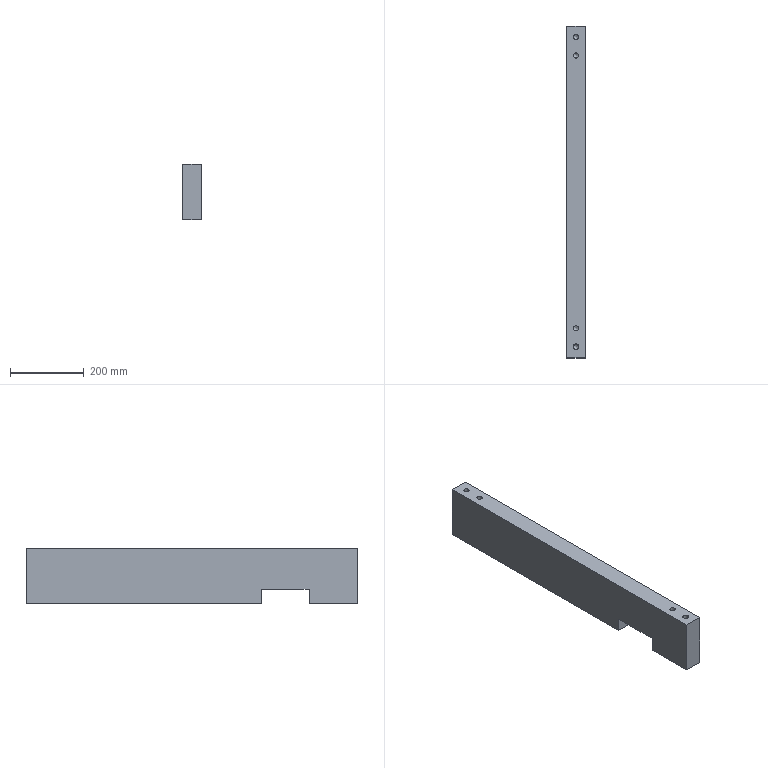Part | STEP file | 1_id762_x_t | 1 solid | 23 faces | box 50 x 900 x 149.325 mm | volume 6424966 mm3 | plane 10 | cone 7 | cylinder 6 | commonest cylinder face diameters 14 x3 10.716 x2 13.495 x1